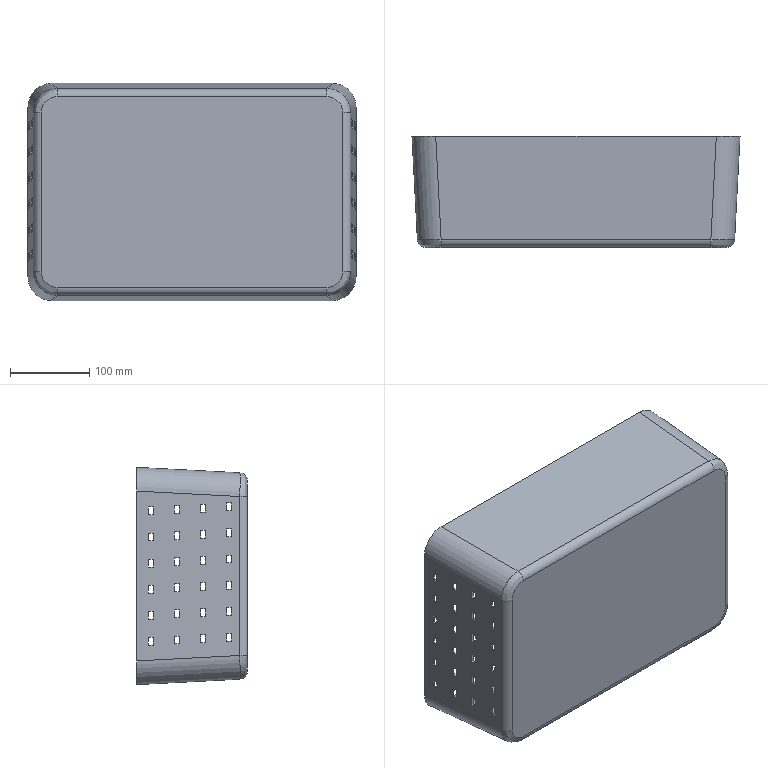Part | SolidWorks | features Fillet 2, Extrusion 1, ICE 1, LPattern 1, Shell 1 | 1 solid | 227 faces | box 414.674 x 140 x 274.674 mm | volume 549320 mm3 | plane 203 | cylinder 16 | spline 8 | commonest cylinder face diameters 16 x4 20 x4 56 x4 60 x4